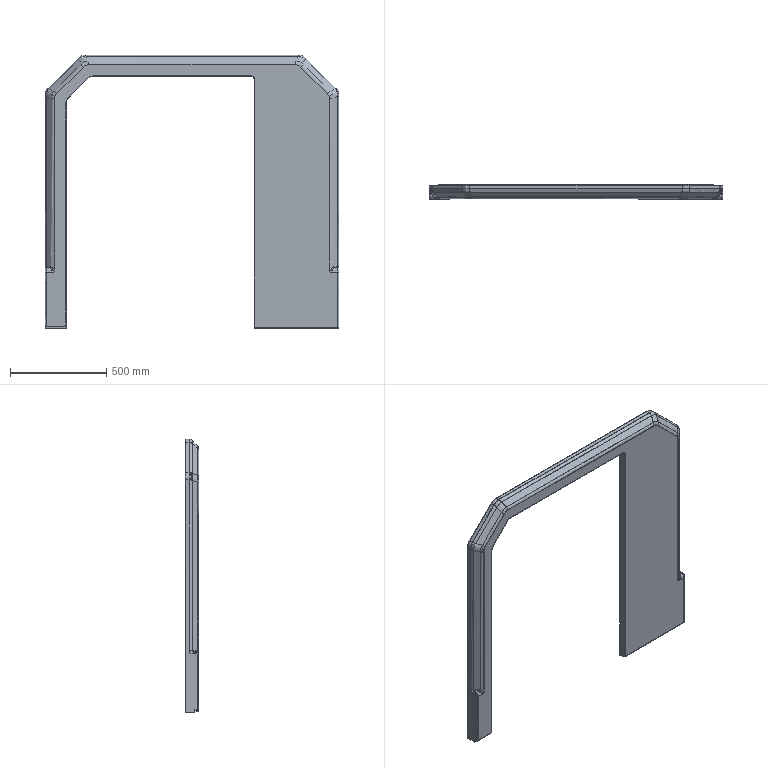Part | NX | features BREP 2 | 3 solids | 281 faces | box 1528 x 70.834 x 1423 mm | volume 4361637 mm3 | spline 131 | plane 104 | cylinder 34 | cone 12 | commonest cylinder face diameters 6 x8 9 x8 2 x6 8 x4 10 x4 13 x4